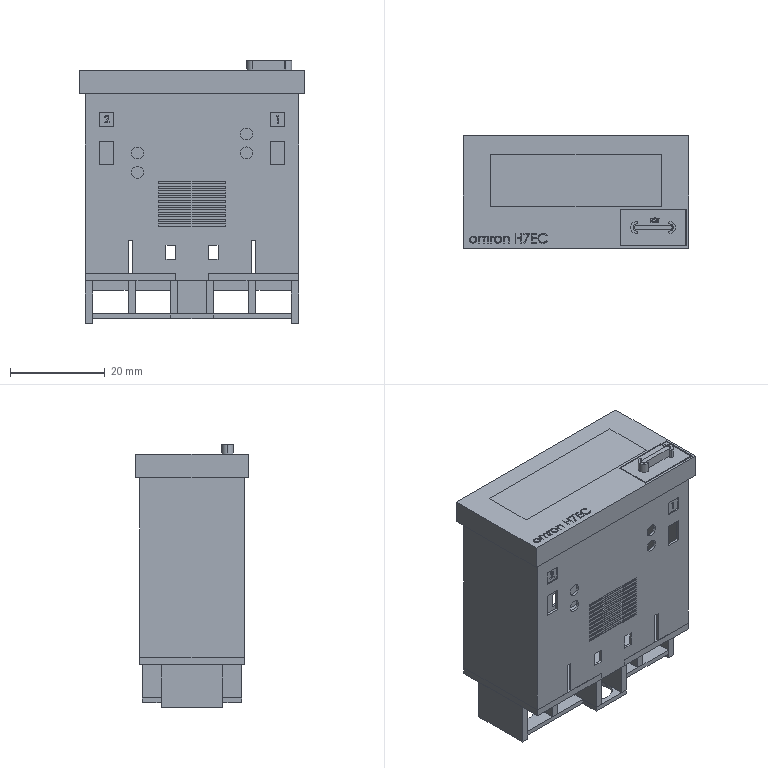Part | STEP file | OMRON H7EC | 13 solids | 527 faces | box 47.6 x 23.8 x 55.5 mm | volume 8164 mm3 | plane 400 | spline 75 | cylinder 52 | commonest cylinder face diameters 4 x16 6.5 x12 2.5 x11 0.5 x6 1 x4 1.5 x3